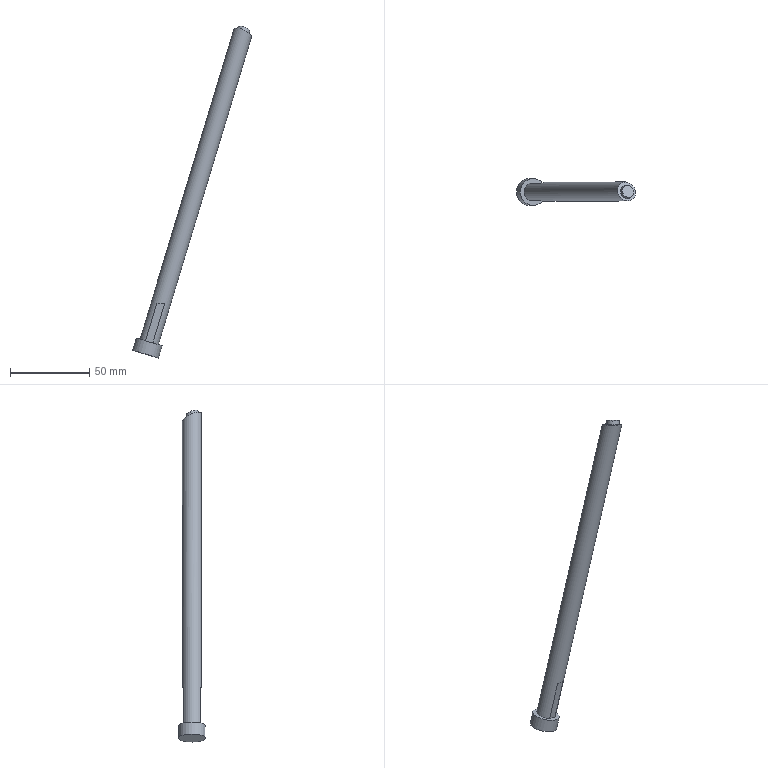Part | STEP file | solid 98 | 1 solid | 12 faces | box 74.766 x 17 x 208.871 mm | volume 24808 mm3 | plane 7 | cylinder 3 | spline 1 | other 1 | commonest cylinder face diameters 8.04 x1 12 x1 17 x1